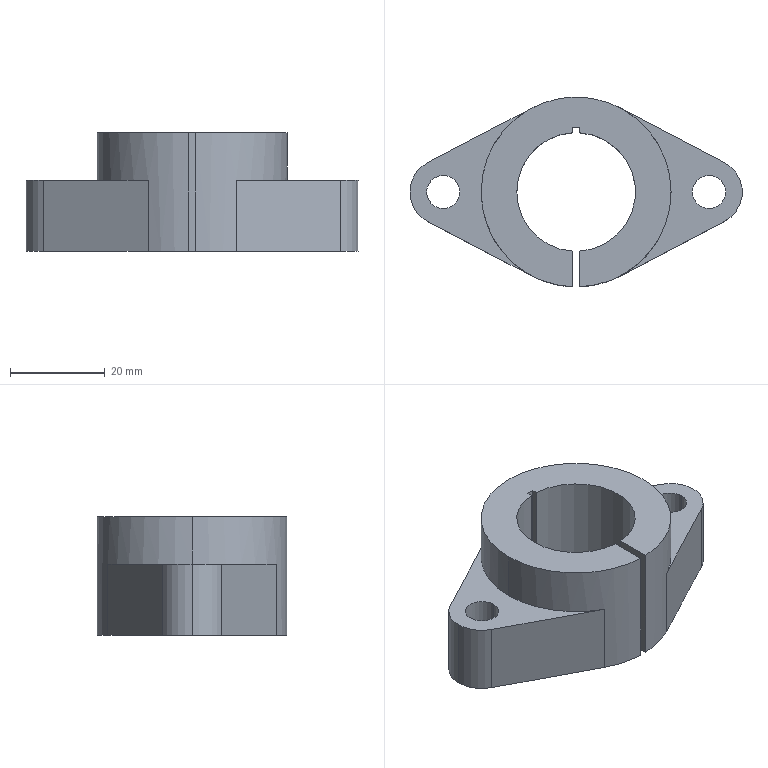Part | STEP file | Open retaining ring | 1 solid | 26 faces | box 70 x 39.986 x 25 mm | volume 26299 mm3 | cylinder 13 | plane 13 | commonest cylinder face diameters 7 x4 14 x3 25 x3 40 x3